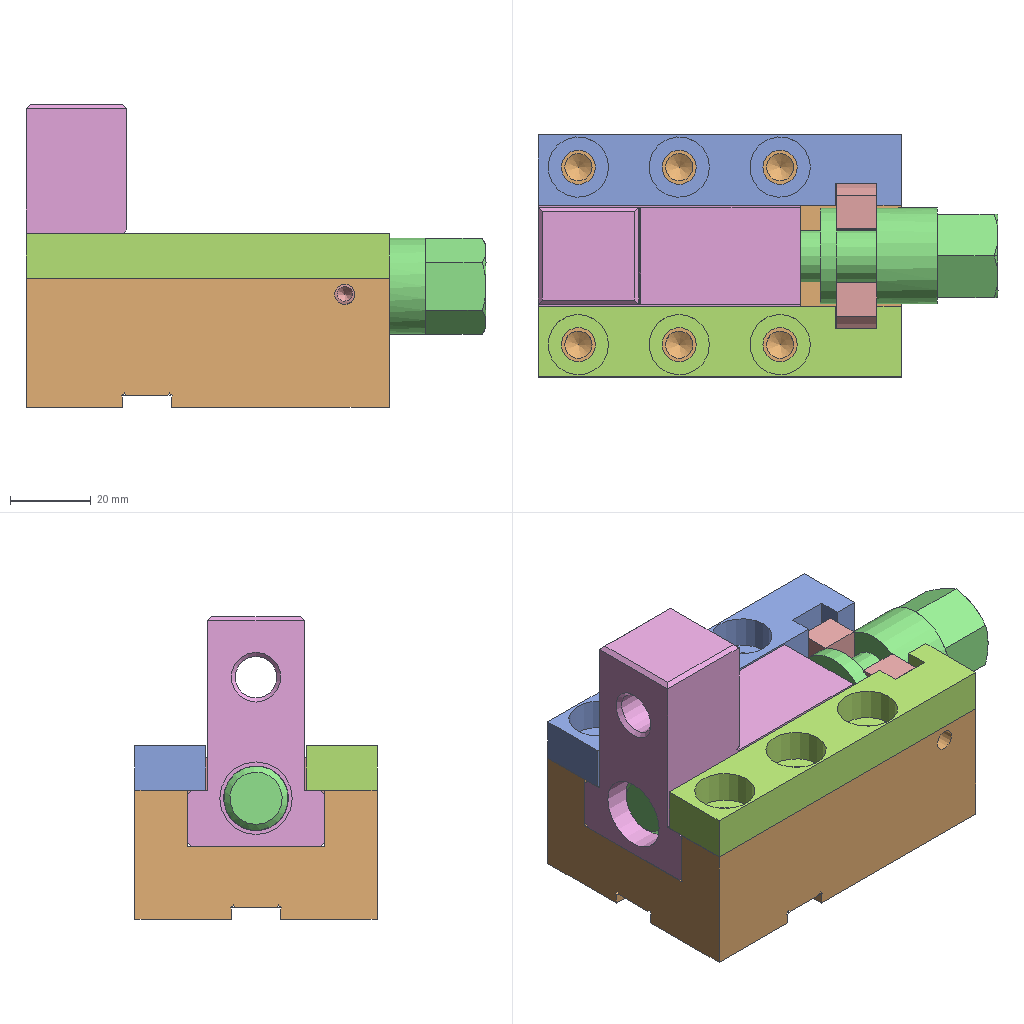Assembly | NX | 7 different items | 7 placed | box 114 x 60 x 75 mm
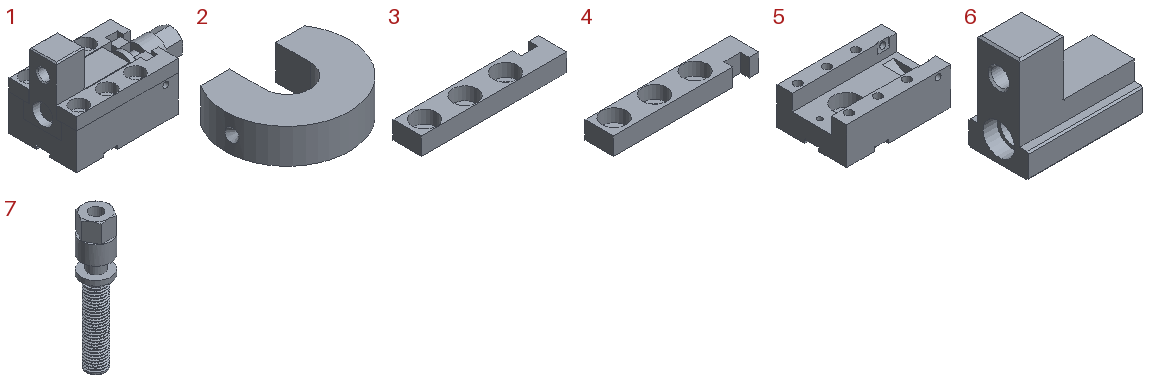Parts list (item | quantity | size | volume | features):
1 | x1 | 114 x 60 x 75 mm | 223844 mm3 | features DATUM_CSYS 37, SKETCH 30, EXTRUDE 22, EXTRACT_FACE 14, EXTRACT_STRING 12, HOLE PACKAGE 12, SIMPLE HOLE 12, SYMBOLIC_THREAD 12, Instance Feature 10, CYLINDER 9, BLOCK 7, CHAMFER 5, Pattern Feature 4, CONE 2, RECT_SLOT 2, SKIN 2, BLEND 1, CPROJ 1, DATUM_ON_PATH 1, DATUM_PLANE 1, MIRROR_SET 1, THREADS 1, TRIM BODY 1
2 | x1 | 36.001 x 28 x 10 mm | 6442 mm3 | features DATUM_CSYS 4, CONE 2, SKETCH 2, EXTRUDE 1, MIRROR_SET 1
3 | x1 | 90 x 17.5 x 11 mm | 11956 mm3 | features EXTRACT_STRING 6, EXTRUDE 6, EXTRACT_FACE 3, DATUM_CSYS 2, Instance Feature 2, BLOCK 1, Pattern Feature 1, RECT_SLOT 1, SKETCH 1
4 | x1 | 90 x 17.5 x 11 mm | 11956 mm3 | features EXTRACT_STRING 6, EXTRUDE 6, EXTRACT_FACE 3, DATUM_CSYS 2, Instance Feature 2, BLOCK 1, Pattern Feature 1, RECT_SLOT 1, SKETCH 1
5 | x1 | 90 x 60 x 32 mm | 114243 mm3 | features DATUM_CSYS 20, SKETCH 19, HOLE PACKAGE 9, SIMPLE HOLE 9, SYMBOLIC_THREAD 9, EXTRACT_FACE 8, EXTRUDE 7, Instance Feature 6, BLOCK 2, CYLINDER 2, Pattern Feature 2, BLEND 1, CPROJ 1
6 | x1 | 65 x 34 x 57 mm | 53379 mm3 | features DATUM_CSYS 5, CHAMFER 4, SKETCH 4, BLOCK 3, CYLINDER 2, HOLE PACKAGE 2, SIMPLE HOLE 2, SYMBOLIC_THREAD 2, EXTRUDE 1
7 | x1 | 23.8 x 23.8 x 110 mm | 24209 mm3 | features CYLINDER 5, DATUM_CSYS 4, SKETCH 3, SKIN 2, CHAMFER 1, DATUM_ON_PATH 1, DATUM_PLANE 1, EXTRUDE 1, HOLE PACKAGE 1, SIMPLE HOLE 1, SYMBOLIC_THREAD 1, THREADS 1, TRIM BODY 1
Mates (type | each side: item.copy, entity, surface, feature):
Fix | 5.1 component | 2 times
Touch | 2.1 face plane Extrude(2) | 5.1 face plane Cylinder(8)
Touch | 2.1 face cylinder Extrude(2) | 5.1 face cylinder Cylinder(7)
Touch | 7.1 face plane Cylinder(5) | 2.1 face plane Extrude(2)
Touch | 4.1 edge | 5.1 face plane Block(1)
Touch | 4.1 face cylinder Extrude(4) | 5.1 face cylinder Pattern Feature [Linear] (12) / Instance[0][1]
Touch | 3.1 face plane Block(1) | 5.1 face plane Block(1)
Touch | 3.1 face cylinder Extrude(3) | 5.1 face cylinder M8 x 1.25 Threaded Hole(10)
Touch | 6.1 face plane Block(1) | 5.1 face plane Block(2) | 2 times
Touch | 6.1 face plane Block(1) | 5.1 face plane Block(1)